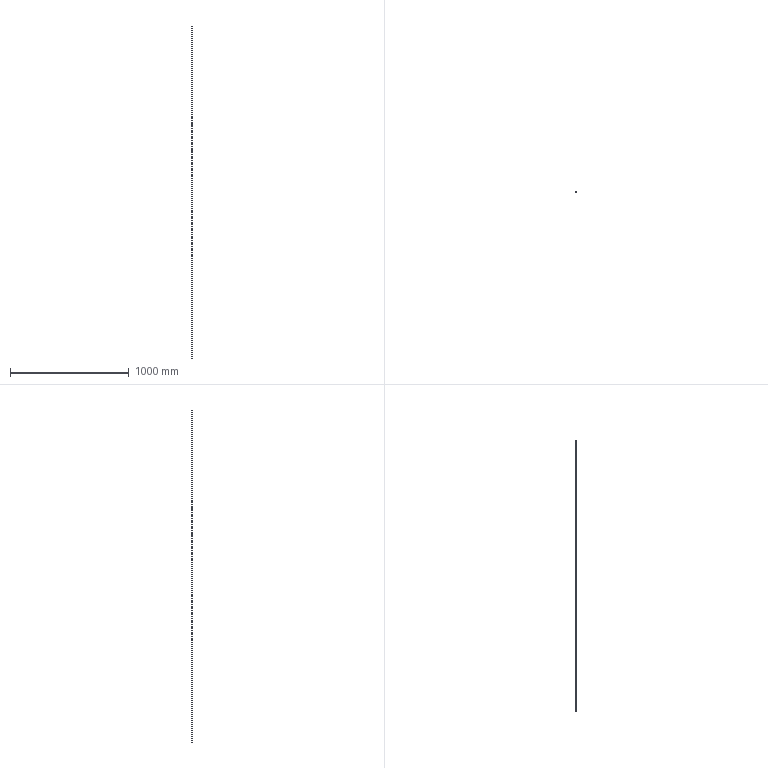Part | STEP file | JIS G 3191A - 6-2 | 1 solid | 3 faces | box 4 x 4 x 2800 mm | volume 35186 mm3 | plane 2 | cylinder 1 | commonest cylinder face diameters 4 x1
STEP:
#1=CARTESIAN_POINT('',(0.,0.,0.));
#2=DIRECTION('',(0.,0.,1.));
#3=DIRECTION('',(1.,0.,0.));
#4=AXIS2_PLACEMENT_3D('',#1,#2,#3);
#5=CARTESIAN_POINT('',(2.,0.,2800.));
#6=VERTEX_POINT('',#5);
#7=CARTESIAN_POINT('',(0.,0.,2800.));
#8=DIRECTION('',(0.,0.,-1.));
#9=DIRECTION('',(-1.,0.,0.));
#10=AXIS2_PLACEMENT_3D('',#7,#8,#9);
#11=CIRCLE('',#10,2.);
#12=CARTESIAN_POINT('',(0.,0.,0.));
#13=DIRECTION('',(0.,0.,1.));
#14=DIRECTION('',(-1.,0.,0.));
#15=AXIS2_PLACEMENT_3D('',#12,#13,#14);
#16=CYLINDRICAL_SURFACE('',#15,2.);
#17=CARTESIAN_POINT('',(12.566,2800.));
#18=DIRECTION('',(-1.,0.));
#19=VECTOR('',#18,1.);
#20=LINE('',#17,#19);
#21=(GEOMETRIC_REPRESENTATION_CONTEXT(2)PARAMETRIC_REPRESENTATION_CONTEXT()REPRESENTATION_CONTEXT('',''));
#22=DEFINITIONAL_REPRESENTATION('',(#20),#21);
#23=PCURVE('',#16,#22);
#24=CARTESIAN_POINT('',(0.,0.,2800.));
#25=DIRECTION('',(0.,0.,1.));
#26=DIRECTION('',(1.,0.,0.));
#27=AXIS2_PLACEMENT_3D('',#24,#25,#26);
#28=PLANE('',#27);
#29=CARTESIAN_POINT('',(-2.,0.));
#30=CARTESIAN_POINT('',(-2.,3.464));
#31=CARTESIAN_POINT('',(1.,1.732));
#32=CARTESIAN_POINT('',(4.,0.));
#33=CARTESIAN_POINT('',(1.,-1.732));
#34=CARTESIAN_POINT('',(-2.,-3.464));
#35=CARTESIAN_POINT('',(-2.,0.));
#36=(BOUNDED_CURVE()B_SPLINE_CURVE(2,(#29,#30,#31,#32,#33,#34,#35),.UNSPECIFIED.,.T.,.F.)B_SPLINE_CURVE_WITH_KNOTS((1,2,2,2,2,1),(-2.094,0.,2.094,4.189,6.283,8.378),.UNSPECIFIED.)CURVE()GEOMETRIC_REPRESENTATION_ITEM()RATIONAL_B_SPLINE_CURVE((1.,0.5,1.,0.5,1.,0.5,1.))REPRESENTATION_ITEM(''));
#37=(GEOMETRIC_REPRESENTATION_CONTEXT(2)PARAMETRIC_REPRESENTATION_CONTEXT()REPRESENTATION_CONTEXT('',''));
#38=DEFINITIONAL_REPRESENTATION('',(#36),#37);
#39=PCURVE('',#28,#38);
#40=SURFACE_CURVE('',#11,(#23,#39),.PCURVE_S1.);
#41=EDGE_CURVE('',#6,#6,#40,.T.);
#42=ORIENTED_EDGE('',*,*,#41,.T.);
#43=CARTESIAN_POINT('',(2.,0.,0.));
#44=VERTEX_POINT('',#43);
#45=CARTESIAN_POINT('',(2.,0.,0.));
#46=CARTESIAN_POINT('',(2.,0.,2800.));
#47=B_SPLINE_CURVE_WITH_KNOTS('',1,(#45,#46),.UNSPECIFIED.,.F.,.F.,(2,2),(0.,2800.),.PIECEWISE_BEZIER_KNOTS.);
#48=CARTESIAN_POINT('',(3.142,0.));
#49=DIRECTION('',(0.,1.));
#50=VECTOR('',#49,1.);
#51=LINE('',#48,#50);
#52=(GEOMETRIC_REPRESENTATION_CONTEXT(2)PARAMETRIC_REPRESENTATION_CONTEXT()REPRESENTATION_CONTEXT('',''));
#53=DEFINITIONAL_REPRESENTATION('',(#51),#52);
#54=PCURVE('',#16,#53);
#55=CARTESIAN_POINT('',(9.425,0.));
#56=DIRECTION('',(0.,1.));
#57=VECTOR('',#56,1.);
#58=LINE('',#55,#57);
#59=(GEOMETRIC_REPRESENTATION_CONTEXT(2)PARAMETRIC_REPRESENTATION_CONTEXT()REPRESENTATION_CONTEXT('',''));
#60=DEFINITIONAL_REPRESENTATION('',(#58),#59);
#61=PCURVE('',#16,#60);
#62=SEAM_CURVE('',#47,(#54,#61),.PCURVE_S1.);
#63=EDGE_CURVE('',#44,#6,#62,.T.);
#64=ORIENTED_EDGE('',*,*,#63,.F.);
#65=CARTESIAN_POINT('',(0.,0.,0.));
#66=DIRECTION('',(0.,0.,-1.));
#67=DIRECTION('',(-1.,0.,0.));
#68=AXIS2_PLACEMENT_3D('',#65,#66,#67);
#69=CIRCLE('',#68,2.);
#70=CARTESIAN_POINT('',(12.566,0.));
#71=DIRECTION('',(-1.,0.));
#72=VECTOR('',#71,1.);
#73=LINE('',#70,#72);
#74=(GEOMETRIC_REPRESENTATION_CONTEXT(2)PARAMETRIC_REPRESENTATION_CONTEXT()REPRESENTATION_CONTEXT('',''));
#75=DEFINITIONAL_REPRESENTATION('',(#73),#74);
#76=PCURVE('',#16,#75);
#77=CARTESIAN_POINT('',(0.,0.,0.));
#78=DIRECTION('',(0.,0.,1.));
#79=DIRECTION('',(1.,0.,0.));
#80=AXIS2_PLACEMENT_3D('',#77,#78,#79);
#81=PLANE('',#80);
#82=CARTESIAN_POINT('',(-2.,0.));
#83=CARTESIAN_POINT('',(-2.,3.464));
#84=CARTESIAN_POINT('',(1.,1.732));
#85=CARTESIAN_POINT('',(4.,0.));
#86=CARTESIAN_POINT('',(1.,-1.732));
#87=CARTESIAN_POINT('',(-2.,-3.464));
#88=CARTESIAN_POINT('',(-2.,0.));
#89=(BOUNDED_CURVE()B_SPLINE_CURVE(2,(#82,#83,#84,#85,#86,#87,#88),.UNSPECIFIED.,.T.,.F.)B_SPLINE_CURVE_WITH_KNOTS((1,2,2,2,2,1),(-2.094,0.,2.094,4.189,6.283,8.378),.UNSPECIFIED.)CURVE()GEOMETRIC_REPRESENTATION_ITEM()RATIONAL_B_SPLINE_CURVE((1.,0.5,1.,0.5,1.,0.5,1.))REPRESENTATION_ITEM(''));
#90=(GEOMETRIC_REPRESENTATION_CONTEXT(2)PARAMETRIC_REPRESENTATION_CONTEXT()REPRESENTATION_CONTEXT('',''));
#91=DEFINITIONAL_REPRESENTATION('',(#89),#90);
#92=PCURVE('',#81,#91);
#93=SURFACE_CURVE('',#69,(#76,#92),.PCURVE_S1.);
#94=EDGE_CURVE('',#44,#44,#93,.T.);
#95=ORIENTED_EDGE('',*,*,#94,.F.);
#96=ORIENTED_EDGE('',*,*,#63,.T.);
#97=EDGE_LOOP('',(#42,#64,#95,#96));
#98=FACE_BOUND('',#97,.T.);
#99=ADVANCED_FACE('',(#98),#16,.T.);
#100=ORIENTED_EDGE('',*,*,#94,.T.);
#101=EDGE_LOOP('',(#100));
#102=FACE_BOUND('',#101,.T.);
#103=ADVANCED_FACE('',(#102),#81,.F.);
#104=ORIENTED_EDGE('',*,*,#41,.F.);
#105=EDGE_LOOP('',(#104));
#106=FACE_BOUND('',#105,.T.);
#107=ADVANCED_FACE('',(#106),#28,.T.);
#108=CLOSED_SHELL('',(#99,#103,#107));
#109=MANIFOLD_SOLID_BREP('',#108);
#110=(LENGTH_UNIT()NAMED_UNIT(*)SI_UNIT(.MILLI.,.METRE.));
#111=UNCERTAINTY_MEASURE_WITH_UNIT(LENGTH_MEASURE(0.00001),#110,'','');
#112=(NAMED_UNIT(*)PLANE_ANGLE_UNIT()SI_UNIT($,.RADIAN.));
#113=(NAMED_UNIT(*)SI_UNIT($,.STERADIAN.)SOLID_ANGLE_UNIT());
#114=(GEOMETRIC_REPRESENTATION_CONTEXT(3)GLOBAL_UNCERTAINTY_ASSIGNED_CONTEXT((#111))GLOBAL_UNIT_ASSIGNED_CONTEXT((#110,#112,#113))REPRESENTATION_CONTEXT('',''));
#115=ADVANCED_BREP_SHAPE_REPRESENTATION('',(#4,#109),#114);